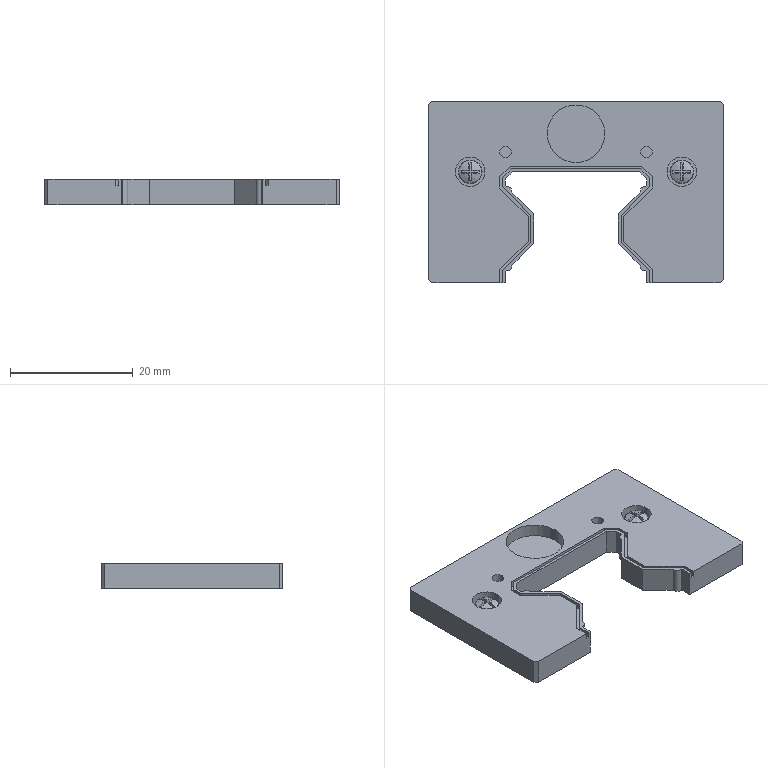Part | STEP file | 2026.6.15-Main Assembly图.sldasm-Part-22 | 1 solid | 117 faces | box 48 x 29.585 x 4.175 mm | volume 4340 mm3 | plane 87 | cylinder 22 | torus 6 | sphere 2 | commonest cylinder face diameters 1.629 x8 1.92 x4 3.84 x4 4.8 x4 9.4 x2